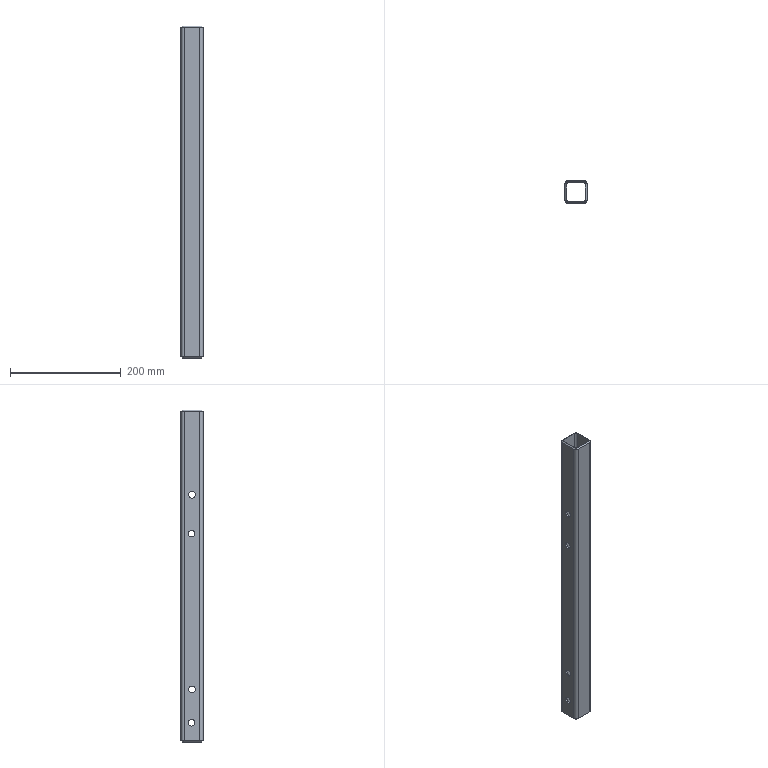Part | STEP file | DIN 59 410 - 40x40x2.9-600_2 | 1 solid | 42 faces | box 40 x 40 x 600 mm | volume 241926 mm3 | plane 18 | cylinder 16 | cone 8 | commonest cylinder face diameters 12.2 x8 5.8 x4 11.6 x4